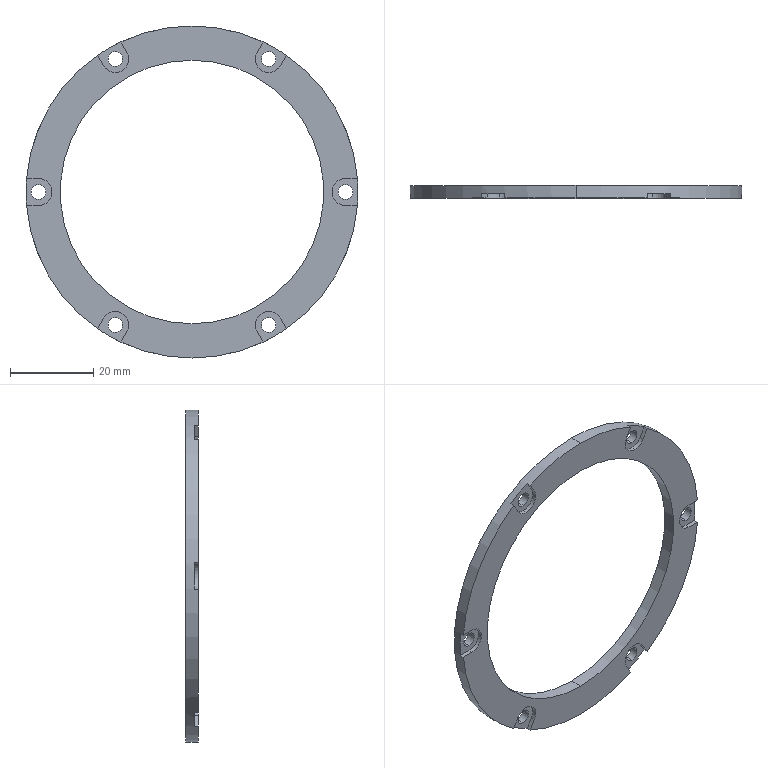Part | SolidWorks | features CirPattern 3, ICE 2, Cut 1, Extrusion 1 | 1 solid | 44 faces | box 80 x 3 x 80 mm | volume 5249 mm3 | cylinder 24 | plane 20 | commonest cylinder face diameters 3.5 x12 6.5 x8 63.5 x2 80 x2
STEP:
#1=CARTESIAN_POINT('',(0.,3.,-31.75));
#2=VERTEX_POINT('',#1);
#3=CARTESIAN_POINT('',(0.,3.,31.75));
#4=VERTEX_POINT('',#3);
#5=CARTESIAN_POINT('',(0.,3.,0.));
#6=DIRECTION('',(0.,1.,0.));
#7=DIRECTION('',(0.,0.,1.));
#8=AXIS2_PLACEMENT_3D('',#5,#6,#7);
#9=CIRCLE('',#8,31.75);
#10=EDGE_CURVE('',#2,#4,#9,.T.);
#11=ORIENTED_EDGE('',*,*,#10,.T.);
#12=CARTESIAN_POINT('',(0.,0.,31.75));
#13=VERTEX_POINT('',#12);
#14=CARTESIAN_POINT('',(0.,3.,31.75));
#15=DIRECTION('',(0.,-1.,0.));
#16=VECTOR('',#15,1000.);
#17=LINE('',#14,#16);
#18=EDGE_CURVE('',#4,#13,#17,.T.);
#19=ORIENTED_EDGE('',*,*,#18,.T.);
#20=CARTESIAN_POINT('',(0.,0.,-31.75));
#21=VERTEX_POINT('',#20);
#22=CARTESIAN_POINT('',(0.,0.,0.));
#23=DIRECTION('',(0.,1.,0.));
#24=DIRECTION('',(0.,0.,1.));
#25=AXIS2_PLACEMENT_3D('',#22,#23,#24);
#26=CIRCLE('',#25,31.75);
#27=EDGE_CURVE('',#21,#13,#26,.T.);
#28=ORIENTED_EDGE('',*,*,#27,.F.);
#29=CARTESIAN_POINT('',(0.,3.,-31.75));
#30=DIRECTION('',(0.,-1.,0.));
#31=VECTOR('',#30,1000.);
#32=LINE('',#29,#31);
#33=EDGE_CURVE('',#2,#21,#32,.T.);
#34=ORIENTED_EDGE('',*,*,#33,.F.);
#35=EDGE_LOOP('',(#11,#19,#28,#34));
#36=FACE_OUTER_BOUND('',#35,.T.);
#37=CARTESIAN_POINT('',(0.,3.,0.));
#38=DIRECTION('',(0.,-1.,0.));
#39=DIRECTION('',(0.,0.,-1.));
#40=AXIS2_PLACEMENT_3D('',#37,#38,#39);
#41=CYLINDRICAL_SURFACE('',#40,31.75);
#42=ADVANCED_FACE('',(#36),#41,.F.);
#43=CARTESIAN_POINT('',(0.,3.,40.));
#44=VERTEX_POINT('',#43);
#45=CARTESIAN_POINT('',(0.,3.,-40.));
#46=VERTEX_POINT('',#45);
#47=CARTESIAN_POINT('',(0.,3.,0.));
#48=DIRECTION('',(0.,1.,0.));
#49=DIRECTION('',(0.,0.,1.));
#50=AXIS2_PLACEMENT_3D('',#47,#48,#49);
#51=CIRCLE('',#50,40.);
#52=EDGE_CURVE('',#44,#46,#51,.T.);
#53=ORIENTED_EDGE('',*,*,#52,.F.);
#54=CARTESIAN_POINT('',(0.,0.,40.));
#55=VERTEX_POINT('',#54);
#56=CARTESIAN_POINT('',(0.,3.,40.));
#57=DIRECTION('',(0.,-1.,0.));
#58=VECTOR('',#57,1000.);
#59=LINE('',#56,#58);
#60=EDGE_CURVE('',#44,#55,#59,.T.);
#61=ORIENTED_EDGE('',*,*,#60,.T.);
#62=CARTESIAN_POINT('',(17.119,0.,36.151));
#63=VERTEX_POINT('',#62);
#64=CARTESIAN_POINT('',(0.,0.,0.));
#65=DIRECTION('',(0.,1.,0.));
#66=DIRECTION('',(0.,0.,1.));
#67=AXIS2_PLACEMENT_3D('',#64,#65,#66);
#68=CIRCLE('',#67,40.);
#69=EDGE_CURVE('',#55,#63,#68,.T.);
#70=ORIENTED_EDGE('',*,*,#69,.T.);
#71=CARTESIAN_POINT('',(17.119,1.,36.151));
#72=VERTEX_POINT('',#71);
#73=CARTESIAN_POINT('',(17.119,3.,36.151));
#74=DIRECTION('',(0.,1.,0.));
#75=VECTOR('',#74,1000.);
#76=LINE('',#73,#75);
#77=EDGE_CURVE('',#63,#72,#76,.T.);
#78=ORIENTED_EDGE('',*,*,#77,.T.);
#79=CARTESIAN_POINT('',(22.748,1.,32.901));
#80=VERTEX_POINT('',#79);
#81=CARTESIAN_POINT('',(0.,1.,0.));
#82=DIRECTION('',(0.,-1.,0.));
#83=DIRECTION('',(0.,0.,-1.));
#84=AXIS2_PLACEMENT_3D('',#81,#82,#83);
#85=CIRCLE('',#84,40.);
#86=EDGE_CURVE('',#80,#72,#85,.T.);
#87=ORIENTED_EDGE('',*,*,#86,.F.);
#88=CARTESIAN_POINT('',(22.748,0.,32.901));
#89=VERTEX_POINT('',#88);
#90=CARTESIAN_POINT('',(22.748,3.,32.901));
#91=DIRECTION('',(0.,-1.,0.));
#92=VECTOR('',#91,1000.);
#93=LINE('',#90,#92);
#94=EDGE_CURVE('',#80,#89,#93,.T.);
#95=ORIENTED_EDGE('',*,*,#94,.T.);
#96=CARTESIAN_POINT('',(39.868,0.,3.25));
#97=VERTEX_POINT('',#96);
#98=CARTESIAN_POINT('',(0.,0.,0.));
#99=DIRECTION('',(0.,1.,0.));
#100=DIRECTION('',(0.,0.,1.));
#101=AXIS2_PLACEMENT_3D('',#98,#99,#100);
#102=CIRCLE('',#101,40.);
#103=EDGE_CURVE('',#89,#97,#102,.T.);
#104=ORIENTED_EDGE('',*,*,#103,.T.);
#105=CARTESIAN_POINT('',(39.868,1.,3.25));
#106=VERTEX_POINT('',#105);
#107=CARTESIAN_POINT('',(39.868,3.,3.25));
#108=DIRECTION('',(0.,1.,0.));
#109=VECTOR('',#108,1000.);
#110=LINE('',#107,#109);
#111=EDGE_CURVE('',#97,#106,#110,.T.);
#112=ORIENTED_EDGE('',*,*,#111,.T.);
#113=CARTESIAN_POINT('',(39.868,1.,-3.25));
#114=VERTEX_POINT('',#113);
#115=CARTESIAN_POINT('',(0.,1.,0.));
#116=DIRECTION('',(0.,-1.,0.));
#117=DIRECTION('',(0.,0.,-1.));
#118=AXIS2_PLACEMENT_3D('',#115,#116,#117);
#119=CIRCLE('',#118,40.);
#120=EDGE_CURVE('',#114,#106,#119,.T.);
#121=ORIENTED_EDGE('',*,*,#120,.F.);
#122=CARTESIAN_POINT('',(39.868,0.,-3.25));
#123=VERTEX_POINT('',#122);
#124=CARTESIAN_POINT('',(39.868,3.,-3.25));
#125=DIRECTION('',(0.,-1.,0.));
#126=VECTOR('',#125,1000.);
#127=LINE('',#124,#126);
#128=EDGE_CURVE('',#114,#123,#127,.T.);
#129=ORIENTED_EDGE('',*,*,#128,.T.);
#130=CARTESIAN_POINT('',(22.748,0.,-32.901));
#131=VERTEX_POINT('',#130);
#132=CARTESIAN_POINT('',(0.,0.,0.));
#133=DIRECTION('',(0.,1.,0.));
#134=DIRECTION('',(0.,0.,1.));
#135=AXIS2_PLACEMENT_3D('',#132,#133,#134);
#136=CIRCLE('',#135,40.);
#137=EDGE_CURVE('',#123,#131,#136,.T.);
#138=ORIENTED_EDGE('',*,*,#137,.T.);
#139=CARTESIAN_POINT('',(22.748,1.,-32.901));
#140=VERTEX_POINT('',#139);
#141=CARTESIAN_POINT('',(22.748,3.,-32.901));
#142=DIRECTION('',(0.,1.,0.));
#143=VECTOR('',#142,1000.);
#144=LINE('',#141,#143);
#145=EDGE_CURVE('',#131,#140,#144,.T.);
#146=ORIENTED_EDGE('',*,*,#145,.T.);
#147=CARTESIAN_POINT('',(17.119,1.,-36.151));
#148=VERTEX_POINT('',#147);
#149=CARTESIAN_POINT('',(0.,1.,0.));
#150=DIRECTION('',(0.,-1.,0.));
#151=DIRECTION('',(0.,0.,-1.));
#152=AXIS2_PLACEMENT_3D('',#149,#150,#151);
#153=CIRCLE('',#152,40.);
#154=EDGE_CURVE('',#148,#140,#153,.T.);
#155=ORIENTED_EDGE('',*,*,#154,.F.);
#156=CARTESIAN_POINT('',(17.119,0.,-36.151));
#157=VERTEX_POINT('',#156);
#158=CARTESIAN_POINT('',(17.119,3.,-36.151));
#159=DIRECTION('',(0.,-1.,0.));
#160=VECTOR('',#159,1000.);
#161=LINE('',#158,#160);
#162=EDGE_CURVE('',#148,#157,#161,.T.);
#163=ORIENTED_EDGE('',*,*,#162,.T.);
#164=CARTESIAN_POINT('',(0.,0.,-40.));
#165=VERTEX_POINT('',#164);
#166=CARTESIAN_POINT('',(0.,0.,0.));
#167=DIRECTION('',(0.,1.,0.));
#168=DIRECTION('',(0.,0.,1.));
#169=AXIS2_PLACEMENT_3D('',#166,#167,#168);
#170=CIRCLE('',#169,40.);
#171=EDGE_CURVE('',#157,#165,#170,.T.);
#172=ORIENTED_EDGE('',*,*,#171,.T.);
#173=CARTESIAN_POINT('',(0.,3.,-40.));
#174=DIRECTION('',(0.,-1.,0.));
#175=VECTOR('',#174,1000.);
#176=LINE('',#173,#175);
#177=EDGE_CURVE('',#46,#165,#176,.T.);
#178=ORIENTED_EDGE('',*,*,#177,.F.);
#179=EDGE_LOOP('',(#53,#61,#70,#78,#87,#95,#104,#112,#121,#129,#138,#146,#155,#163,#172,#178));
#180=FACE_OUTER_BOUND('',#179,.T.);
#181=CARTESIAN_POINT('',(0.,3.,0.));
#182=DIRECTION('',(0.,-1.,0.));
#183=DIRECTION('',(0.,0.,-1.));
#184=AXIS2_PLACEMENT_3D('',#181,#182,#183);
#185=CYLINDRICAL_SURFACE('',#184,40.);
#186=ADVANCED_FACE('',(#180),#185,.T.);
#187=CARTESIAN_POINT('',(18.5,3.,33.793));
#188=VERTEX_POINT('',#187);
#189=CARTESIAN_POINT('',(18.5,3.,30.293));
#190=VERTEX_POINT('',#189);
#191=CARTESIAN_POINT('',(18.5,3.,32.043));
#192=DIRECTION('',(0.,-1.,0.));
#193=DIRECTION('',(0.866,0.,-0.5));
#194=AXIS2_PLACEMENT_3D('',#191,#192,#193);
#195=CIRCLE('',#194,1.75);
#196=EDGE_CURVE('',#188,#190,#195,.T.);
#197=ORIENTED_EDGE('',*,*,#196,.F.);
#198=CARTESIAN_POINT('',(18.5,1.,33.793));
#199=VERTEX_POINT('',#198);
#200=CARTESIAN_POINT('',(18.5,3.,33.793));
#201=DIRECTION('',(0.,-1.,0.));
#202=VECTOR('',#201,1000.);
#203=LINE('',#200,#202);
#204=EDGE_CURVE('',#188,#199,#203,.T.);
#205=ORIENTED_EDGE('',*,*,#204,.T.);
#206=CARTESIAN_POINT('',(18.5,1.,30.293));
#207=VERTEX_POINT('',#206);
#208=CARTESIAN_POINT('',(18.5,1.,32.043));
#209=DIRECTION('',(0.,1.,0.));
#210=DIRECTION('',(0.,0.,-1.));
#211=AXIS2_PLACEMENT_3D('',#208,#209,#210);
#212=CIRCLE('',#211,1.75);
#213=EDGE_CURVE('',#207,#199,#212,.T.);
#214=ORIENTED_EDGE('',*,*,#213,.F.);
#215=CARTESIAN_POINT('',(18.5,3.,30.293));
#216=DIRECTION('',(0.,-1.,0.));
#217=VECTOR('',#216,1000.);
#218=LINE('',#215,#217);
#219=EDGE_CURVE('',#190,#207,#218,.T.);
#220=ORIENTED_EDGE('',*,*,#219,.F.);
#221=EDGE_LOOP('',(#197,#205,#214,#220));
#222=FACE_OUTER_BOUND('',#221,.T.);
#223=CARTESIAN_POINT('',(18.5,3.,32.043));
#224=DIRECTION('',(0.,-1.,0.));
#225=DIRECTION('',(0.,0.,-1.));
#226=AXIS2_PLACEMENT_3D('',#223,#224,#225);
#227=CYLINDRICAL_SURFACE('',#226,1.75);
#228=ADVANCED_FACE('',(#222),#227,.F.);
#229=CARTESIAN_POINT('',(-18.5,3.,33.793));
#230=VERTEX_POINT('',#229);
#231=CARTESIAN_POINT('',(-18.5,3.,30.293));
#232=VERTEX_POINT('',#231);
#233=CARTESIAN_POINT('',(-18.5,3.,32.043));
#234=DIRECTION('',(0.,-1.,0.));
#235=DIRECTION('',(0.866,0.,0.5));
#236=AXIS2_PLACEMENT_3D('',#233,#234,#235);
#237=CIRCLE('',#236,1.75);
#238=EDGE_CURVE('',#230,#232,#237,.T.);
#239=ORIENTED_EDGE('',*,*,#238,.F.);
#240=CARTESIAN_POINT('',(-18.5,1.,33.793));
#241=VERTEX_POINT('',#240);
#242=CARTESIAN_POINT('',(-18.5,3.,33.793));
#243=DIRECTION('',(0.,-1.,0.));
#244=VECTOR('',#243,1000.);
#245=LINE('',#242,#244);
#246=EDGE_CURVE('',#230,#241,#245,.T.);
#247=ORIENTED_EDGE('',*,*,#246,.T.);
#248=CARTESIAN_POINT('',(-18.5,1.,30.293));
#249=VERTEX_POINT('',#248);
#250=CARTESIAN_POINT('',(-18.5,1.,32.043));
#251=DIRECTION('',(0.,1.,0.));
#252=DIRECTION('',(0.,0.,-1.));
#253=AXIS2_PLACEMENT_3D('',#250,#251,#252);
#254=CIRCLE('',#253,1.75);
#255=EDGE_CURVE('',#249,#241,#254,.T.);
#256=ORIENTED_EDGE('',*,*,#255,.F.);
#257=CARTESIAN_POINT('',(-18.5,3.,30.293));
#258=DIRECTION('',(0.,-1.,0.));
#259=VECTOR('',#258,1000.);
#260=LINE('',#257,#259);
#261=EDGE_CURVE('',#232,#249,#260,.T.);
#262=ORIENTED_EDGE('',*,*,#261,.F.);
#263=EDGE_LOOP('',(#239,#247,#256,#262));
#264=FACE_OUTER_BOUND('',#263,.T.);
#265=CARTESIAN_POINT('',(-18.5,3.,32.043));
#266=DIRECTION('',(0.,-1.,0.));
#267=DIRECTION('',(0.,0.,-1.));
#268=AXIS2_PLACEMENT_3D('',#265,#266,#267);
#269=CYLINDRICAL_SURFACE('',#268,1.75);
#270=ADVANCED_FACE('',(#264),#269,.F.);
#271=CARTESIAN_POINT('',(-37.,3.,1.75));
#272=VERTEX_POINT('',#271);
#273=CARTESIAN_POINT('',(-37.,3.,-1.75));
#274=VERTEX_POINT('',#273);
#275=CARTESIAN_POINT('',(-37.,3.,0.));
#276=DIRECTION('',(0.,-1.,0.));
#277=DIRECTION('',(0.,0.,1.));
#278=AXIS2_PLACEMENT_3D('',#275,#276,#277);
#279=CIRCLE('',#278,1.75);
#280=EDGE_CURVE('',#272,#274,#279,.T.);
#281=ORIENTED_EDGE('',*,*,#280,.F.);
#282=CARTESIAN_POINT('',(-37.,1.,1.75));
#283=VERTEX_POINT('',#282);
#284=CARTESIAN_POINT('',(-37.,3.,1.75));
#285=DIRECTION('',(0.,-1.,0.));
#286=VECTOR('',#285,1000.);
#287=LINE('',#284,#286);
#288=EDGE_CURVE('',#272,#283,#287,.T.);
#289=ORIENTED_EDGE('',*,*,#288,.T.);
#290=CARTESIAN_POINT('',(-37.,1.,-1.75));
#291=VERTEX_POINT('',#290);
#292=CARTESIAN_POINT('',(-37.,1.,0.));
#293=DIRECTION('',(0.,1.,0.));
#294=DIRECTION('',(0.,0.,-1.));
#295=AXIS2_PLACEMENT_3D('',#292,#293,#294);
#296=CIRCLE('',#295,1.75);
#297=EDGE_CURVE('',#291,#283,#296,.T.);
#298=ORIENTED_EDGE('',*,*,#297,.F.);
#299=CARTESIAN_POINT('',(-37.,3.,-1.75));
#300=DIRECTION('',(0.,-1.,0.));
#301=VECTOR('',#300,1000.);
#302=LINE('',#299,#301);
#303=EDGE_CURVE('',#274,#291,#302,.T.);
#304=ORIENTED_EDGE('',*,*,#303,.F.);
#305=EDGE_LOOP('',(#281,#289,#298,#304));
#306=FACE_OUTER_BOUND('',#305,.T.);
#307=CARTESIAN_POINT('',(-37.,3.,0.));
#308=DIRECTION('',(0.,-1.,0.));
#309=DIRECTION('',(0.,0.,-1.));
#310=AXIS2_PLACEMENT_3D('',#307,#308,#309);
#311=CYLINDRICAL_SURFACE('',#310,1.75);
#312=ADVANCED_FACE('',(#306),#311,.F.);
#313=CARTESIAN_POINT('',(-18.5,3.,-30.293));
#314=VERTEX_POINT('',#313);
#315=CARTESIAN_POINT('',(-18.5,3.,-33.793));
#316=VERTEX_POINT('',#315);
#317=CARTESIAN_POINT('',(-18.5,3.,-32.043));
#318=DIRECTION('',(0.,-1.,0.));
#319=DIRECTION('',(-0.866,0.,0.5));
#320=AXIS2_PLACEMENT_3D('',#317,#318,#319);
#321=CIRCLE('',#320,1.75);
#322=EDGE_CURVE('',#314,#316,#321,.T.);
#323=ORIENTED_EDGE('',*,*,#322,.F.);
#324=CARTESIAN_POINT('',(-18.5,1.,-30.293));
#325=VERTEX_POINT('',#324);
#326=CARTESIAN_POINT('',(-18.5,3.,-30.293));
#327=DIRECTION('',(0.,-1.,0.));
#328=VECTOR('',#327,1000.);
#329=LINE('',#326,#328);
#330=EDGE_CURVE('',#314,#325,#329,.T.);
#331=ORIENTED_EDGE('',*,*,#330,.T.);
#332=CARTESIAN_POINT('',(-18.5,1.,-33.793));
#333=VERTEX_POINT('',#332);
#334=CARTESIAN_POINT('',(-18.5,1.,-32.043));
#335=DIRECTION('',(0.,1.,0.));
#336=DIRECTION('',(0.,0.,-1.));
#337=AXIS2_PLACEMENT_3D('',#334,#335,#336);
#338=CIRCLE('',#337,1.75);
#339=EDGE_CURVE('',#333,#325,#338,.T.);
#340=ORIENTED_EDGE('',*,*,#339,.F.);
#341=CARTESIAN_POINT('',(-18.5,3.,-33.793));
#342=DIRECTION('',(0.,-1.,0.));
#343=VECTOR('',#342,1000.);
#344=LINE('',#341,#343);
#345=EDGE_CURVE('',#316,#333,#344,.T.);
#346=ORIENTED_EDGE('',*,*,#345,.F.);
#347=EDGE_LOOP('',(#323,#331,#340,#346));
#348=FACE_OUTER_BOUND('',#347,.T.);
#349=CARTESIAN_POINT('',(-18.5,3.,-32.043));
#350=DIRECTION('',(0.,-1.,0.));
#351=DIRECTION('',(0.,0.,-1.));
#352=AXIS2_PLACEMENT_3D('',#349,#350,#351);
#353=CYLINDRICAL_SURFACE('',#352,1.75);
#354=ADVANCED_FACE('',(#348),#353,.F.);
#355=CARTESIAN_POINT('',(18.5,3.,-30.293));
#356=VERTEX_POINT('',#355);
#357=CARTESIAN_POINT('',(18.5,3.,-33.793));
#358=VERTEX_POINT('',#357);
#359=CARTESIAN_POINT('',(18.5,3.,-32.043));
#360=DIRECTION('',(0.,-1.,0.));
#361=DIRECTION('',(-0.866,0.,-0.5));
#362=AXIS2_PLACEMENT_3D('',#359,#360,#361);
#363=CIRCLE('',#362,1.75);
#364=EDGE_CURVE('',#356,#358,#363,.T.);
#365=ORIENTED_EDGE('',*,*,#364,.F.);
#366=CARTESIAN_POINT('',(18.5,1.,-30.293));
#367=VERTEX_POINT('',#366);
#368=CARTESIAN_POINT('',(18.5,3.,-30.293));
#369=DIRECTION('',(0.,-1.,0.));
#370=VECTOR('',#369,1000.);
#371=LINE('',#368,#370);
#372=EDGE_CURVE('',#356,#367,#371,.T.);
#373=ORIENTED_EDGE('',*,*,#372,.T.);
#374=CARTESIAN_POINT('',(18.5,1.,-33.793));
#375=VERTEX_POINT('',#374);
#376=CARTESIAN_POINT('',(18.5,1.,-32.043));
#377=DIRECTION('',(0.,1.,0.));
#378=DIRECTION('',(0.,0.,-1.));
#379=AXIS2_PLACEMENT_3D('',#376,#377,#378);
#380=CIRCLE('',#379,1.75);
#381=EDGE_CURVE('',#375,#367,#380,.T.);
#382=ORIENTED_EDGE('',*,*,#381,.F.);
#383=CARTESIAN_POINT('',(18.5,3.,-33.793));
#384=DIRECTION('',(0.,-1.,0.));
#385=VECTOR('',#384,1000.);
#386=LINE('',#383,#385);
#387=EDGE_CURVE('',#358,#375,#386,.T.);
#388=ORIENTED_EDGE('',*,*,#387,.F.);
#389=EDGE_LOOP('',(#365,#373,#382,#388));
#390=FACE_OUTER_BOUND('',#389,.T.);
#391=CARTESIAN_POINT('',(18.5,3.,-32.043));
#392=DIRECTION('',(0.,-1.,0.));
#393=DIRECTION('',(0.,0.,-1.));
#394=AXIS2_PLACEMENT_3D('',#391,#392,#393);
#395=CYLINDRICAL_SURFACE('',#394,1.75);
#396=ADVANCED_FACE('',(#390),#395,.F.);
#397=CARTESIAN_POINT('',(37.,3.,1.75));
#398=VERTEX_POINT('',#397);
#399=CARTESIAN_POINT('',(37.,3.,-1.75));
#400=VERTEX_POINT('',#399);
#401=CARTESIAN_POINT('',(37.,3.,0.));
#402=DIRECTION('',(0.,-1.,0.));
#403=DIRECTION('',(0.,0.,-1.));
#404=AXIS2_PLACEMENT_3D('',#401,#402,#403);
#405=CIRCLE('',#404,1.75);
#406=EDGE_CURVE('',#398,#400,#405,.T.);
#407=ORIENTED_EDGE('',*,*,#406,.F.);
#408=CARTESIAN_POINT('',(37.,1.,1.75));
#409=VERTEX_POINT('',#408);
#410=CARTESIAN_POINT('',(37.,3.,1.75));
#411=DIRECTION('',(0.,-1.,0.));
#412=VECTOR('',#411,1000.);
#413=LINE('',#410,#412);
#414=EDGE_CURVE('',#398,#409,#413,.T.);
#415=ORIENTED_EDGE('',*,*,#414,.T.);
#416=CARTESIAN_POINT('',(37.,1.,-1.75));
#417=VERTEX_POINT('',#416);
#418=CARTESIAN_POINT('',(37.,1.,0.));
#419=DIRECTION('',(0.,1.,0.));
#420=DIRECTION('',(0.,0.,-1.));
#421=AXIS2_PLACEMENT_3D('',#418,#419,#420);
#422=CIRCLE('',#421,1.75);
#423=EDGE_CURVE('',#417,#409,#422,.T.);
#424=ORIENTED_EDGE('',*,*,#423,.F.);
#425=CARTESIAN_POINT('',(37.,3.,-1.75));
#426=DIRECTION('',(0.,-1.,0.));
#427=VECTOR('',#426,1000.);
#428=LINE('',#425,#427);
#429=EDGE_CURVE('',#400,#417,#428,.T.);
#430=ORIENTED_EDGE('',*,*,#429,.F.);
#431=EDGE_LOOP('',(#407,#415,#424,#430));
#432=FACE_OUTER_BOUND('',#431,.T.);
#433=CARTESIAN_POINT('',(37.,3.,0.));
#434=DIRECTION('',(0.,-1.,0.));
#435=DIRECTION('',(0.,0.,-1.));
#436=AXIS2_PLACEMENT_3D('',#433,#434,#435);
#437=CYLINDRICAL_SURFACE('',#436,1.75);
#438=ADVANCED_FACE('',(#432),#437,.F.);
#439=CARTESIAN_POINT('',(18.5,1.,28.793));
#440=VERTEX_POINT('',#439);
#441=CARTESIAN_POINT('',(21.315,1.,30.418));
#442=VERTEX_POINT('',#441);
#443=CARTESIAN_POINT('',(18.5,1.,32.043));
#444=DIRECTION('',(0.,-1.,0.));
#445=DIRECTION('',(0.,0.,-1.));
#446=AXIS2_PLACEMENT_3D('',#443,#444,#445);
#447=CIRCLE('',#446,3.25);
#448=EDGE_CURVE('',#440,#442,#447,.T.);
#449=ORIENTED_EDGE('',*,*,#448,.F.);
#450=CARTESIAN_POINT('',(18.5,0.,28.793));
#451=VERTEX_POINT('',#450);
#452=CARTESIAN_POINT('',(18.5,1.,28.793));
#453=DIRECTION('',(0.,-1.,0.));
#454=VECTOR('',#453,1000.);
#455=LINE('',#452,#454);
#456=EDGE_CURVE('',#440,#451,#455,.T.);
#457=ORIENTED_EDGE('',*,*,#456,.T.);
#458=CARTESIAN_POINT('',(21.315,0.,30.418));
#459=VERTEX_POINT('',#458);
#460=CARTESIAN_POINT('',(18.5,0.,32.043));
#461=DIRECTION('',(0.,-1.,0.));
#462=DIRECTION('',(0.,0.,-1.));
#463=AXIS2_PLACEMENT_3D('',#460,#461,#462);
#464=CIRCLE('',#463,3.25);
#465=EDGE_CURVE('',#451,#459,#464,.T.);
#466=ORIENTED_EDGE('',*,*,#465,.T.);
#467=CARTESIAN_POINT('',(21.315,10.69,30.418));
#468=DIRECTION('',(0.,-1.,0.));
#469=VECTOR('',#468,1000.);
#470=LINE('',#467,#469);
#471=EDGE_CURVE('',#442,#459,#470,.T.);
#472=ORIENTED_EDGE('',*,*,#471,.F.);
#473=EDGE_LOOP('',(#449,#457,#466,#472));
#474=FACE_OUTER_BOUND('',#473,.T.);
#475=CARTESIAN_POINT('',(18.5,1.,32.043));
#476=DIRECTION('',(0.,-1.,0.));
#477=DIRECTION('',(0.,0.,-1.));
#478=AXIS2_PLACEMENT_3D('',#475,#476,#477);
#479=CYLINDRICAL_SURFACE('',#478,3.25);
#480=ADVANCED_FACE('',(#474),#479,.F.);
#481=CARTESIAN_POINT('',(-18.5,1.,28.793));
#482=VERTEX_POINT('',#481);
#483=CARTESIAN_POINT('',(-15.685,1.,33.668));
#484=VERTEX_POINT('',#483);
#485=CARTESIAN_POINT('',(-18.5,1.,32.043));
#486=DIRECTION('',(0.,-1.,0.));
#487=DIRECTION('',(0.866,0.,-0.5));
#488=AXIS2_PLACEMENT_3D('',#485,#486,#487);
#489=CIRCLE('',#488,3.25);
#490=EDGE_CURVE('',#482,#484,#489,.T.);
#491=ORIENTED_EDGE('',*,*,#490,.F.);
#492=CARTESIAN_POINT('',(-18.5,0.,28.793));
#493=VERTEX_POINT('',#492);
#494=CARTESIAN_POINT('',(-18.5,1.,28.793));
#495=DIRECTION('',(0.,-1.,0.));
#496=VECTOR('',#495,1000.);
#497=LINE('',#494,#496);
#498=EDGE_CURVE('',#482,#493,#497,.T.);
#499=ORIENTED_EDGE('',*,*,#498,.T.);
#500=CARTESIAN_POINT('',(-15.685,0.,33.668));
#501=VERTEX_POINT('',#500);
#502=CARTESIAN_POINT('',(-18.5,0.,32.043));
#503=DIRECTION('',(0.,-1.,0.));
#504=DIRECTION('',(0.866,0.,-0.5));
#505=AXIS2_PLACEMENT_3D('',#502,#503,#504);
#506=CIRCLE('',#505,3.25);
#507=EDGE_CURVE('',#493,#501,#506,.T.);
#508=ORIENTED_EDGE('',*,*,#507,.T.);
#509=CARTESIAN_POINT('',(-15.685,10.69,33.668));
#510=DIRECTION('',(0.,-1.,0.));
#511=VECTOR('',#510,1000.);
#512=LINE('',#509,#511);
#513=EDGE_CURVE('',#484,#501,#512,.T.);
#514=ORIENTED_EDGE('',*,*,#513,.F.);
#515=EDGE_LOOP('',(#491,#499,#508,#514));
#516=FACE_OUTER_BOUND('',#515,.T.);
#517=CARTESIAN_POINT('',(-18.5,1.,32.043));
#518=DIRECTION('',(0.,-1.,0.));
#519=DIRECTION('',(0.,0.,-1.));
#520=AXIS2_PLACEMENT_3D('',#517,#518,#519);
#521=CYLINDRICAL_SURFACE('',#520,3.25);
#522=ADVANCED_FACE('',(#516),#521,.F.);
#523=CARTESIAN_POINT('',(21.315,1.,-30.418));
#524=VERTEX_POINT('',#523);
#525=CARTESIAN_POINT('',(21.315,0.,-30.418));
#526=VERTEX_POINT('',#525);
#527=CARTESIAN_POINT('',(21.315,10.69,-30.418));
#528=DIRECTION('',(0.,-1.,0.));
#529=VECTOR('',#528,1000.);
#530=LINE('',#527,#529);
#531=EDGE_CURVE('',#524,#526,#530,.T.);
#532=ORIENTED_EDGE('',*,*,#531,.T.);
#533=CARTESIAN_POINT('',(15.685,0.,-33.668));
#534=VERTEX_POINT('',#533);
#535=CARTESIAN_POINT('',(18.5,0.,-32.043));
#536=DIRECTION('',(0.,-1.,0.));
#537=DIRECTION('',(-0.866,0.,0.5));
#538=AXIS2_PLACEMENT_3D('',#535,#536,#537);
#539=CIRCLE('',#538,3.25);
#540=EDGE_CURVE('',#526,#534,#539,.T.);
#541=ORIENTED_EDGE('',*,*,#540,.T.);
#542=CARTESIAN_POINT('',(15.685,1.,-33.668));
#543=VERTEX_POINT('',#542);
#544=CARTESIAN_POINT('',(15.685,10.69,-33.668));
#545=DIRECTION('',(0.,-1.,0.));
#546=VECTOR('',#545,1000.);
#547=LINE('',#544,#546);
#548=EDGE_CURVE('',#543,#534,#547,.T.);
#549=ORIENTED_EDGE('',*,*,#548,.F.);
#550=CARTESIAN_POINT('',(18.5,1.,-32.043));
#551=DIRECTION('',(0.,-1.,0.));
#552=DIRECTION('',(-0.866,0.,0.5));
#553=AXIS2_PLACEMENT_3D('',#550,#551,#552);
#554=CIRCLE('',#553,3.25);
#555=EDGE_CURVE('',#524,#543,#554,.T.);
#556=ORIENTED_EDGE('',*,*,#555,.F.);
#557=EDGE_LOOP('',(#532,#541,#549,#556));
#558=FACE_OUTER_BOUND('',#557,.T.);
#559=CARTESIAN_POINT('',(18.5,1.,-32.043));
#560=DIRECTION('',(0.,-1.,0.));
#561=DIRECTION('',(0.,0.,-1.));
#562=AXIS2_PLACEMENT_3D('',#559,#560,#561);
#563=CYLINDRICAL_SURFACE('',#562,3.25);
#564=ADVANCED_FACE('',(#558),#563,.F.);
#565=CARTESIAN_POINT('',(-15.685,1.,-33.668));
#566=VERTEX_POINT('',#565);
#567=CARTESIAN_POINT('',(-15.685,0.,-33.668));
#568=VERTEX_POINT('',#567);
#569=CARTESIAN_POINT('',(-15.685,10.69,-33.668));
#570=DIRECTION('',(0.,-1.,0.));
#571=VECTOR('',#570,1000.);
#572=LINE('',#569,#571);
#573=EDGE_CURVE('',#566,#568,#572,.T.);
#574=ORIENTED_EDGE('',*,*,#573,.T.);
#575=CARTESIAN_POINT('',(-21.315,0.,-30.418));
#576=VERTEX_POINT('',#575);
#577=CARTESIAN_POINT('',(-18.5,0.,-32.043));
#578=DIRECTION('',(0.,-1.,0.));
#579=DIRECTION('',(0.,0.,1.));
#580=AXIS2_PLACEMENT_3D('',#577,#578,#579);
#581=CIRCLE('',#580,3.25);
#582=EDGE_CURVE('',#568,#576,#581,.T.);
#583=ORIENTED_EDGE('',*,*,#582,.T.);
#584=CARTESIAN_POINT('',(-21.315,1.,-30.418));
#585=VERTEX_POINT('',#584);
#586=CARTESIAN_POINT('',(-21.315,10.69,-30.418));
#587=DIRECTION('',(0.,-1.,0.));
#588=VECTOR('',#587,1000.);
#589=LINE('',#586,#588);
#590=EDGE_CURVE('',#585,#576,#589,.T.);
#591=ORIENTED_EDGE('',*,*,#590,.F.);
#592=CARTESIAN_POINT('',(-18.5,1.,-32.043));
#593=DIRECTION('',(0.,-1.,0.));
#594=DIRECTION('',(0.,0.,1.));
#595=AXIS2_PLACEMENT_3D('',#592,#593,#594);
#596=CIRCLE('',#595,3.25);
#597=EDGE_CURVE('',#566,#585,#596,.T.);
#598=ORIENTED_EDGE('',*,*,#597,.F.);
#599=EDGE_LOOP('',(#574,#583,#591,#598));
#600=FACE_OUTER_BOUND('',#599,.T.);
#601=CARTESIAN_POINT('',(-18.5,1.,-32.043));
#602=DIRECTION('',(0.,-1.,0.));
#603=DIRECTION('',(0.,0.,-1.));
#604=AXIS2_PLACEMENT_3D('',#601,#602,#603);
#605=CYLINDRICAL_SURFACE('',#604,3.25);
#606=ADVANCED_FACE('',(#600),#605,.F.);
#607=CARTESIAN_POINT('',(-37.,1.,-3.25));
#608=VERTEX_POINT('',#607);
#609=CARTESIAN_POINT('',(-37.,0.,-3.25));
#610=VERTEX_POINT('',#609);
#611=CARTESIAN_POINT('',(-37.,8.382,-3.25));
#612=DIRECTION('',(0.,-1.,0.));
#613=VECTOR('',#612,1000.);
#614=LINE('',#611,#613);
#615=EDGE_CURVE('',#608,#610,#614,.T.);
#616=ORIENTED_EDGE('',*,*,#615,.T.);
#617=CARTESIAN_POINT('',(-37.,0.,3.25));
#618=VERTEX_POINT('',#617);
#619=CARTESIAN_POINT('',(-37.,0.,0.));
#620=DIRECTION('',(0.,-1.,0.));
#621=DIRECTION('',(0.866,0.,0.5));
#622=AXIS2_PLACEMENT_3D('',#619,#620,#621);
#623=CIRCLE('',#622,3.25);
#624=EDGE_CURVE('',#610,#618,#623,.T.);
#625=ORIENTED_EDGE('',*,*,#624,.T.);
#626=CARTESIAN_POINT('',(-37.,1.,3.25));
#627=VERTEX_POINT('',#626);
#628=CARTESIAN_POINT('',(-37.,8.382,3.25));
#629=DIRECTION('',(0.,-1.,0.));
#630=VECTOR('',#629,1000.);
#631=LINE('',#628,#630);
#632=EDGE_CURVE('',#627,#618,#631,.T.);
#633=ORIENTED_EDGE('',*,*,#632,.F.);
#634=CARTESIAN_POINT('',(-37.,1.,0.));
#635=DIRECTION('',(0.,-1.,0.));
#636=DIRECTION('',(0.866,0.,0.5));
#637=AXIS2_PLACEMENT_3D('',#634,#635,#636);
#638=CIRCLE('',#637,3.25);
#639=EDGE_CURVE('',#608,#627,#638,.T.);
#640=ORIENTED_EDGE('',*,*,#639,.F.);
#641=EDGE_LOOP('',(#616,#625,#633,#640));
#642=FACE_OUTER_BOUND('',#641,.T.);
#643=CARTESIAN_POINT('',(-37.,1.,0.));
#644=DIRECTION('',(0.,-1.,0.));
#645=DIRECTION('',(0.,0.,-1.));
#646=AXIS2_PLACEMENT_3D('',#643,#644,#645);
#647=CYLINDRICAL_SURFACE('',#646,3.25);
#648=ADVANCED_FACE('',(#642),#647,.F.);
#649=ORIENTED_EDGE('',*,*,#498,.F.);
#650=CARTESIAN_POINT('',(-21.315,1.,30.418));
#651=VERTEX_POINT('',#650);
#652=CARTESIAN_POINT('',(-18.5,1.,32.043));
#653=DIRECTION('',(0.,-1.,0.));
#654=DIRECTION('',(0.866,0.,-0.5));
#655=AXIS2_PLACEMENT_3D('',#652,#653,#654);
#656=CIRCLE('',#655,3.25);
#657=EDGE_CURVE('',#651,#482,#656,.T.);
#658=ORIENTED_EDGE('',*,*,#657,.F.);
#659=CARTESIAN_POINT('',(-21.315,0.,30.418));
#660=VERTEX_POINT('',#659);
#661=CARTESIAN_POINT('',(-21.315,10.69,30.418));
#662=DIRECTION('',(0.,-1.,0.));
#663=VECTOR('',#662,1000.);
#664=LINE('',#661,#663);
#665=EDGE_CURVE('',#651,#660,#664,.T.);
#666=ORIENTED_EDGE('',*,*,#665,.T.);
#667=CARTESIAN_POINT('',(-18.5,0.,32.043));
#668=DIRECTION('',(0.,-1.,0.));
#669=DIRECTION('',(0.866,0.,-0.5));
#670=AXIS2_PLACEMENT_3D('',#667,#668,#669);
#671=CIRCLE('',#670,3.25);
#672=EDGE_CURVE('',#660,#493,#671,.T.);
#673=ORIENTED_EDGE('',*,*,#672,.T.);
#674=EDGE_LOOP('',(#649,#658,#666,#673));
#675=FACE_OUTER_BOUND('',#674,.T.);
#676=CARTESIAN_POINT('',(-18.5,1.,32.043));
#677=DIRECTION('',(0.,-1.,0.));
#678=DIRECTION('',(0.,0.,-1.));
#679=AXIS2_PLACEMENT_3D('',#676,#677,#678);
#680=CYLINDRICAL_SURFACE('',#679,3.25);
#681=ADVANCED_FACE('',(#675),#680,.F.);
#682=ORIENTED_EDGE('',*,*,#456,.F.);
#683=CARTESIAN_POINT('',(15.685,1.,33.668));
#684=VERTEX_POINT('',#683);
#685=CARTESIAN_POINT('',(18.5,1.,32.043));
#686=DIRECTION('',(0.,-1.,0.));
#687=DIRECTION('',(0.,0.,-1.));
#688=AXIS2_PLACEMENT_3D('',#685,#686,#687);
#689=CIRCLE('',#688,3.25);
#690=EDGE_CURVE('',#684,#440,#689,.T.);
#691=ORIENTED_EDGE('',*,*,#690,.F.);
#692=CARTESIAN_POINT('',(15.685,0.,33.668));
#693=VERTEX_POINT('',#692);
#694=CARTESIAN_POINT('',(15.685,10.69,33.668));
#695=DIRECTION('',(0.,-1.,0.));
#696=VECTOR('',#695,1000.);
#697=LINE('',#694,#696);
#698=EDGE_CURVE('',#684,#693,#697,.T.);
#699=ORIENTED_EDGE('',*,*,#698,.T.);
#700=CARTESIAN_POINT('',(18.5,0.,32.043));
#701=DIRECTION('',(0.,-1.,0.));
#702=DIRECTION('',(0.,0.,-1.));
#703=AXIS2_PLACEMENT_3D('',#700,#701,#702);
#704=CIRCLE('',#703,3.25);
#705=EDGE_CURVE('',#693,#451,#704,.T.);
#706=ORIENTED_EDGE('',*,*,#705,.T.);
#707=EDGE_LOOP('',(#682,#691,#699,#706));
#708=FACE_OUTER_BOUND('',#707,.T.);
#709=CARTESIAN_POINT('',(18.5,1.,32.043));
#710=DIRECTION('',(0.,-1.,0.));
#711=DIRECTION('',(0.,0.,-1.));
#712=AXIS2_PLACEMENT_3D('',#709,#710,#711);
#713=CYLINDRICAL_SURFACE('',#712,3.25);
#714=ADVANCED_FACE('',(#708),#713,.F.);
#715=CARTESIAN_POINT('',(37.,1.,3.25));
#716=VERTEX_POINT('',#715);
#717=CARTESIAN_POINT('',(37.,0.,3.25));
#718=VERTEX_POINT('',#717);
#719=CARTESIAN_POINT('',(37.,8.382,3.25));
#720=DIRECTION('',(0.,-1.,0.));
#721=VECTOR('',#720,1000.);
#722=LINE('',#719,#721);
#723=EDGE_CURVE('',#716,#718,#722,.T.);
#724=ORIENTED_EDGE('',*,*,#723,.T.);
#725=CARTESIAN_POINT('',(37.,0.,-3.25));
#726=VERTEX_POINT('',#725);
#727=CARTESIAN_POINT('',(37.,0.,0.));
#728=DIRECTION('',(0.,-1.,0.));
#729=DIRECTION('',(-0.866,0.,-0.5));
#730=AXIS2_PLACEMENT_3D('',#727,#728,#729);
#731=CIRCLE('',#730,3.25);
#732=EDGE_CURVE('',#718,#726,#731,.T.);
#733=ORIENTED_EDGE('',*,*,#732,.T.);
#734=CARTESIAN_POINT('',(37.,1.,-3.25));
#735=VERTEX_POINT('',#734);
#736=CARTESIAN_POINT('',(37.,8.382,-3.25));
#737=DIRECTION('',(0.,-1.,0.));
#738=VECTOR('',#737,1000.);
#739=LINE('',#736,#738);
#740=EDGE_CURVE('',#735,#726,#739,.T.);
#741=ORIENTED_EDGE('',*,*,#740,.F.);
#742=CARTESIAN_POINT('',(37.,1.,0.));
#743=DIRECTION('',(0.,-1.,0.));
#744=DIRECTION('',(-0.866,0.,-0.5));
#745=AXIS2_PLACEMENT_3D('',#742,#743,#744);
#746=CIRCLE('',#745,3.25);
#747=EDGE_CURVE('',#716,#735,#746,.T.);
#748=ORIENTED_EDGE('',*,*,#747,.F.);
#749=EDGE_LOOP('',(#724,#733,#741,#748));
#750=FACE_OUTER_BOUND('',#749,.T.);
#751=CARTESIAN_POINT('',(37.,1.,0.));
#752=DIRECTION('',(0.,-1.,0.));
#753=DIRECTION('',(0.,0.,-1.));
#754=AXIS2_PLACEMENT_3D('',#751,#752,#753);
#755=CYLINDRICAL_SURFACE('',#754,3.25);
#756=ADVANCED_FACE('',(#750),#755,.F.);
#757=ORIENTED_EDGE('',*,*,#414,.F.);
#758=CARTESIAN_POINT('',(37.,3.,0.));
#759=DIRECTION('',(0.,-1.,0.));
#760=DIRECTION('',(0.,0.,-1.));
#761=AXIS2_PLACEMENT_3D('',#758,#759,#760);
#762=CIRCLE('',#761,1.75);
#763=EDGE_CURVE('',#400,#398,#762,.T.);
#764=ORIENTED_EDGE('',*,*,#763,.F.);
#765=ORIENTED_EDGE('',*,*,#429,.T.);
#766=CARTESIAN_POINT('',(37.,1.,0.));
#767=DIRECTION('',(0.,1.,0.));
#768=DIRECTION('',(0.,0.,-1.));
#769=AXIS2_PLACEMENT_3D('',#766,#767,#768);
#770=CIRCLE('',#769,1.75);
#771=EDGE_CURVE('',#409,#417,#770,.T.);
#772=ORIENTED_EDGE('',*,*,#771,.F.);
#773=EDGE_LOOP('',(#757,#764,#765,#772));
#774=FACE_OUTER_BOUND('',#773,.T.);
#775=CARTESIAN_POINT('',(37.,3.,0.));
#776=DIRECTION('',(0.,-1.,0.));
#777=DIRECTION('',(0.,0.,-1.));
#778=AXIS2_PLACEMENT_3D('',#775,#776,#777);
#779=CYLINDRICAL_SURFACE('',#778,1.75);
#780=ADVANCED_FACE('',(#774),#779,.F.);
#781=ORIENTED_EDGE('',*,*,#372,.F.);
#782=CARTESIAN_POINT('',(18.5,3.,-32.043));
#783=DIRECTION('',(0.,-1.,0.));
#784=DIRECTION('',(-0.866,0.,-0.5));
#785=AXIS2_PLACEMENT_3D('',#782,#783,#784);
#786=CIRCLE('',#785,1.75);
#787=EDGE_CURVE('',#358,#356,#786,.T.);
#788=ORIENTED_EDGE('',*,*,#787,.F.);
#789=ORIENTED_EDGE('',*,*,#387,.T.);
#790=CARTESIAN_POINT('',(18.5,1.,-32.043));
#791=DIRECTION('',(0.,1.,0.));
#792=DIRECTION('',(0.,0.,-1.));
#793=AXIS2_PLACEMENT_3D('',#790,#791,#792);
#794=CIRCLE('',#793,1.75);
#795=EDGE_CURVE('',#367,#375,#794,.T.);
#796=ORIENTED_EDGE('',*,*,#795,.F.);
#797=EDGE_LOOP('',(#781,#788,#789,#796));
#798=FACE_OUTER_BOUND('',#797,.T.);
#799=CARTESIAN_POINT('',(18.5,3.,-32.043));
#800=DIRECTION('',(0.,-1.,0.));
#801=DIRECTION('',(0.,0.,-1.));
#802=AXIS2_PLACEMENT_3D('',#799,#800,#801);
#803=CYLINDRICAL_SURFACE('',#802,1.75);
#804=ADVANCED_FACE('',(#798),#803,.F.);
#805=ORIENTED_EDGE('',*,*,#330,.F.);
#806=CARTESIAN_POINT('',(-18.5,3.,-32.043));
#807=DIRECTION('',(0.,-1.,0.));
#808=DIRECTION('',(-0.866,0.,0.5));
#809=AXIS2_PLACEMENT_3D('',#806,#807,#808);
#810=CIRCLE('',#809,1.75);
#811=EDGE_CURVE('',#316,#314,#810,.T.);
#812=ORIENTED_EDGE('',*,*,#811,.F.);
#813=ORIENTED_EDGE('',*,*,#345,.T.);
#814=CARTESIAN_POINT('',(-18.5,1.,-32.043));
#815=DIRECTION('',(0.,1.,0.));
#816=DIRECTION('',(0.,0.,-1.));
#817=AXIS2_PLACEMENT_3D('',#814,#815,#816);
#818=CIRCLE('',#817,1.75);
#819=EDGE_CURVE('',#325,#333,#818,.T.);
#820=ORIENTED_EDGE('',*,*,#819,.F.);
#821=EDGE_LOOP('',(#805,#812,#813,#820));
#822=FACE_OUTER_BOUND('',#821,.T.);
#823=CARTESIAN_POINT('',(-18.5,3.,-32.043));
#824=DIRECTION('',(0.,-1.,0.));
#825=DIRECTION('',(0.,0.,-1.));
#826=AXIS2_PLACEMENT_3D('',#823,#824,#825);
#827=CYLINDRICAL_SURFACE('',#826,1.75);
#828=ADVANCED_FACE('',(#822),#827,.F.);
#829=ORIENTED_EDGE('',*,*,#288,.F.);
#830=CARTESIAN_POINT('',(-37.,3.,0.));
#831=DIRECTION('',(0.,-1.,0.));
#832=DIRECTION('',(0.,0.,1.));
#833=AXIS2_PLACEMENT_3D('',#830,#831,#832);
#834=CIRCLE('',#833,1.75);
#835=EDGE_CURVE('',#274,#272,#834,.T.);
#836=ORIENTED_EDGE('',*,*,#835,.F.);
#837=ORIENTED_EDGE('',*,*,#303,.T.);
#838=CARTESIAN_POINT('',(-37.,1.,0.));
#839=DIRECTION('',(0.,1.,0.));
#840=DIRECTION('',(0.,0.,-1.));
#841=AXIS2_PLACEMENT_3D('',#838,#839,#840);
#842=CIRCLE('',#841,1.75);
#843=EDGE_CURVE('',#283,#291,#842,.T.);
#844=ORIENTED_EDGE('',*,*,#843,.F.);
#845=EDGE_LOOP('',(#829,#836,#837,#844));
#846=FACE_OUTER_BOUND('',#845,.T.);
#847=CARTESIAN_POINT('',(-37.,3.,0.));
#848=DIRECTION('',(0.,-1.,0.));
#849=DIRECTION('',(0.,0.,-1.));
#850=AXIS2_PLACEMENT_3D('',#847,#848,#849);
#851=CYLINDRICAL_SURFACE('',#850,1.75);
#852=ADVANCED_FACE('',(#846),#851,.F.);
#853=ORIENTED_EDGE('',*,*,#246,.F.);
#854=CARTESIAN_POINT('',(-18.5,3.,32.043));
#855=DIRECTION('',(0.,-1.,0.));
#856=DIRECTION('',(0.866,0.,0.5));
#857=AXIS2_PLACEMENT_3D('',#854,#855,#856);
#858=CIRCLE('',#857,1.75);
#859=EDGE_CURVE('',#232,#230,#858,.T.);
#860=ORIENTED_EDGE('',*,*,#859,.F.);
#861=ORIENTED_EDGE('',*,*,#261,.T.);
#862=CARTESIAN_POINT('',(-18.5,1.,32.043));
#863=DIRECTION('',(0.,1.,0.));
#864=DIRECTION('',(0.,0.,-1.));
#865=AXIS2_PLACEMENT_3D('',#862,#863,#864);
#866=CIRCLE('',#865,1.75);
#867=EDGE_CURVE('',#241,#249,#866,.T.);
#868=ORIENTED_EDGE('',*,*,#867,.F.);
#869=EDGE_LOOP('',(#853,#860,#861,#868));
#870=FACE_OUTER_BOUND('',#869,.T.);
#871=CARTESIAN_POINT('',(-18.5,3.,32.043));
#872=DIRECTION('',(0.,-1.,0.));
#873=DIRECTION('',(0.,0.,-1.));
#874=AXIS2_PLACEMENT_3D('',#871,#872,#873);
#875=CYLINDRICAL_SURFACE('',#874,1.75);
#876=ADVANCED_FACE('',(#870),#875,.F.);
#877=ORIENTED_EDGE('',*,*,#204,.F.);
#878=CARTESIAN_POINT('',(18.5,3.,32.043));
#879=DIRECTION('',(0.,-1.,0.));
#880=DIRECTION('',(0.866,0.,-0.5));
#881=AXIS2_PLACEMENT_3D('',#878,#879,#880);
#882=CIRCLE('',#881,1.75);
#883=EDGE_CURVE('',#190,#188,#882,.T.);
#884=ORIENTED_EDGE('',*,*,#883,.F.);
#885=ORIENTED_EDGE('',*,*,#219,.T.);
#886=CARTESIAN_POINT('',(18.5,1.,32.043));
#887=DIRECTION('',(0.,1.,0.));
#888=DIRECTION('',(0.,0.,-1.));
#889=AXIS2_PLACEMENT_3D('',#886,#887,#888);
#890=CIRCLE('',#889,1.75);
#891=EDGE_CURVE('',#199,#207,#890,.T.);
#892=ORIENTED_EDGE('',*,*,#891,.F.);
#893=EDGE_LOOP('',(#877,#884,#885,#892));
#894=FACE_OUTER_BOUND('',#893,.T.);
#895=CARTESIAN_POINT('',(18.5,3.,32.043));
#896=DIRECTION('',(0.,-1.,0.));
#897=DIRECTION('',(0.,0.,-1.));
#898=AXIS2_PLACEMENT_3D('',#895,#896,#897);
#899=CYLINDRICAL_SURFACE('',#898,1.75);
#900=ADVANCED_FACE('',(#894),#899,.F.);
#901=ORIENTED_EDGE('',*,*,#787,.T.);
#902=ORIENTED_EDGE('',*,*,#364,.T.);
#903=EDGE_LOOP('',(#901,#902));
#904=FACE_BOUND('',#903,.T.);
#905=ORIENTED_EDGE('',*,*,#811,.T.);
#906=ORIENTED_EDGE('',*,*,#322,.T.);
#907=EDGE_LOOP('',(#905,#906));
#908=FACE_BOUND('',#907,.T.);
#909=ORIENTED_EDGE('',*,*,#835,.T.);
#910=ORIENTED_EDGE('',*,*,#280,.T.);
#911=EDGE_LOOP('',(#909,#910));
#912=FACE_BOUND('',#911,.T.);
#913=ORIENTED_EDGE('',*,*,#859,.T.);
#914=ORIENTED_EDGE('',*,*,#238,.T.);
#915=EDGE_LOOP('',(#913,#914));
#916=FACE_BOUND('',#915,.T.);
#917=ORIENTED_EDGE('',*,*,#883,.T.);
#918=ORIENTED_EDGE('',*,*,#196,.T.);
#919=EDGE_LOOP('',(#917,#918));
#920=FACE_BOUND('',#919,.T.);
#921=ORIENTED_EDGE('',*,*,#763,.T.);
#922=ORIENTED_EDGE('',*,*,#406,.T.);
#923=EDGE_LOOP('',(#921,#922));
#924=FACE_BOUND('',#923,.T.);
#925=CARTESIAN_POINT('',(0.,3.,0.));
#926=DIRECTION('',(0.,1.,0.));
#927=DIRECTION('',(0.,0.,1.));
#928=AXIS2_PLACEMENT_3D('',#925,#926,#927);
#929=CIRCLE('',#928,40.);
#930=EDGE_CURVE('',#46,#44,#929,.T.);
#931=ORIENTED_EDGE('',*,*,#930,.T.);
#932=ORIENTED_EDGE('',*,*,#52,.T.);
#933=EDGE_LOOP('',(#931,#932));
#934=FACE_OUTER_BOUND('',#933,.T.);
#935=ORIENTED_EDGE('',*,*,#10,.F.);
#936=CARTESIAN_POINT('',(0.,3.,0.));
#937=DIRECTION('',(0.,1.,0.));
#938=DIRECTION('',(0.,0.,1.));
#939=AXIS2_PLACEMENT_3D('',#936,#937,#938);
#940=CIRCLE('',#939,31.75);
#941=EDGE_CURVE('',#4,#2,#940,.T.);
#942=ORIENTED_EDGE('',*,*,#941,.F.);
#943=EDGE_LOOP('',(#935,#942));
#944=FACE_BOUND('',#943,.T.);
#945=CARTESIAN_POINT('',(0.,3.,0.));
#946=DIRECTION('',(0.,1.,0.));
#947=DIRECTION('',(0.,0.,1.));
#948=AXIS2_PLACEMENT_3D('',#945,#946,#947);
#949=PLANE('',#948);
#950=ADVANCED_FACE('',(#904,#908,#912,#916,#920,#924,#934,#944),#949,.T.);
#951=ORIENTED_EDGE('',*,*,#540,.F.);
#952=CARTESIAN_POINT('',(23.065,0.,-33.449));
#953=DIRECTION('',(-0.5,0.,0.866));
#954=VECTOR('',#953,1000.);
#955=LINE('',#952,#954);
#956=EDGE_CURVE('',#131,#526,#955,.T.);
#957=ORIENTED_EDGE('',*,*,#956,.F.);
#958=ORIENTED_EDGE('',*,*,#137,.F.);
#959=CARTESIAN_POINT('',(40.5,0.,-3.25));
#960=DIRECTION('',(1.,0.,0.));
#961=VECTOR('',#960,1000.);
#962=LINE('',#959,#961);
#963=EDGE_CURVE('',#726,#123,#962,.T.);
#964=ORIENTED_EDGE('',*,*,#963,.F.);
#965=ORIENTED_EDGE('',*,*,#732,.F.);
#966=CARTESIAN_POINT('',(40.5,0.,3.25));
#967=DIRECTION('',(-1.,0.,0.));
#968=VECTOR('',#967,1000.);
#969=LINE('',#966,#968);
#970=EDGE_CURVE('',#97,#718,#969,.T.);
#971=ORIENTED_EDGE('',*,*,#970,.F.);
#972=ORIENTED_EDGE('',*,*,#103,.F.);
#973=CARTESIAN_POINT('',(23.065,0.,33.449));
#974=DIRECTION('',(0.5,0.,0.866));
#975=VECTOR('',#974,1000.);
#976=LINE('',#973,#975);
#977=EDGE_CURVE('',#459,#89,#976,.T.);
#978=ORIENTED_EDGE('',*,*,#977,.F.);
#979=ORIENTED_EDGE('',*,*,#465,.F.);
#980=ORIENTED_EDGE('',*,*,#705,.F.);
#981=CARTESIAN_POINT('',(17.435,0.,36.699));
#982=DIRECTION('',(-0.5,0.,-0.866));
#983=VECTOR('',#982,1000.);
#984=LINE('',#981,#983);
#985=EDGE_CURVE('',#63,#693,#984,.T.);
#986=ORIENTED_EDGE('',*,*,#985,.F.);
#987=ORIENTED_EDGE('',*,*,#69,.F.);
#988=CARTESIAN_POINT('',(-17.119,0.,36.151));
#989=VERTEX_POINT('',#988);
#990=CARTESIAN_POINT('',(0.,0.,0.));
#991=DIRECTION('',(0.,1.,0.));
#992=DIRECTION('',(0.,0.,1.));
#993=AXIS2_PLACEMENT_3D('',#990,#991,#992);
#994=CIRCLE('',#993,40.);
#995=EDGE_CURVE('',#989,#55,#994,.T.);
#996=ORIENTED_EDGE('',*,*,#995,.F.);
#997=CARTESIAN_POINT('',(-17.435,0.,36.699));
#998=DIRECTION('',(-0.5,0.,0.866));
#999=VECTOR('',#998,1000.);
#1000=LINE('',#997,#999);
#1001=EDGE_CURVE('',#501,#989,#1000,.T.);
#1002=ORIENTED_EDGE('',*,*,#1001,.F.);
#1003=ORIENTED_EDGE('',*,*,#507,.F.);
#1004=ORIENTED_EDGE('',*,*,#672,.F.);
#1005=CARTESIAN_POINT('',(-22.748,0.,32.901));
#1006=VERTEX_POINT('',#1005);
#1007=CARTESIAN_POINT('',(-23.065,0.,33.449));
#1008=DIRECTION('',(0.5,0.,-0.866));
#1009=VECTOR('',#1008,1000.);
#1010=LINE('',#1007,#1009);
#1011=EDGE_CURVE('',#1006,#660,#1010,.T.);
#1012=ORIENTED_EDGE('',*,*,#1011,.F.);
#1013=CARTESIAN_POINT('',(-39.868,0.,3.25));
#1014=VERTEX_POINT('',#1013);
#1015=CARTESIAN_POINT('',(0.,0.,0.));
#1016=DIRECTION('',(0.,1.,0.));
#1017=DIRECTION('',(0.,0.,1.));
#1018=AXIS2_PLACEMENT_3D('',#1015,#1016,#1017);
#1019=CIRCLE('',#1018,40.);
#1020=EDGE_CURVE('',#1014,#1006,#1019,.T.);
#1021=ORIENTED_EDGE('',*,*,#1020,.F.);
#1022=CARTESIAN_POINT('',(-40.5,0.,3.25));
#1023=DIRECTION('',(-1.,0.,0.));
#1024=VECTOR('',#1023,1000.);
#1025=LINE('',#1022,#1024);
#1026=EDGE_CURVE('',#618,#1014,#1025,.T.);
#1027=ORIENTED_EDGE('',*,*,#1026,.F.);
#1028=ORIENTED_EDGE('',*,*,#624,.F.);
#1029=CARTESIAN_POINT('',(-39.868,0.,-3.25));
#1030=VERTEX_POINT('',#1029);
#1031=CARTESIAN_POINT('',(-40.5,0.,-3.25));
#1032=DIRECTION('',(1.,0.,0.));
#1033=VECTOR('',#1032,1000.);
#1034=LINE('',#1031,#1033);
#1035=EDGE_CURVE('',#1030,#610,#1034,.T.);
#1036=ORIENTED_EDGE('',*,*,#1035,.F.);
#1037=CARTESIAN_POINT('',(-22.748,0.,-32.901));
#1038=VERTEX_POINT('',#1037);
#1039=CARTESIAN_POINT('',(0.,0.,0.));
#1040=DIRECTION('',(0.,1.,0.));
#1041=DIRECTION('',(0.,0.,1.));
#1042=AXIS2_PLACEMENT_3D('',#1039,#1040,#1041);
#1043=CIRCLE('',#1042,40.);
#1044=EDGE_CURVE('',#1038,#1030,#1043,.T.);
#1045=ORIENTED_EDGE('',*,*,#1044,.F.);
#1046=CARTESIAN_POINT('',(-23.065,0.,-33.449));
#1047=DIRECTION('',(-0.5,0.,-0.866));
#1048=VECTOR('',#1047,1000.);
#1049=LINE('',#1046,#1048);
#1050=EDGE_CURVE('',#576,#1038,#1049,.T.);
#1051=ORIENTED_EDGE('',*,*,#1050,.F.);
#1052=ORIENTED_EDGE('',*,*,#582,.F.);
#1053=CARTESIAN_POINT('',(-17.119,0.,-36.151));
#1054=VERTEX_POINT('',#1053);
#1055=CARTESIAN_POINT('',(-17.435,0.,-36.699));
#1056=DIRECTION('',(0.5,0.,0.866));
#1057=VECTOR('',#1056,1000.);
#1058=LINE('',#1055,#1057);
#1059=EDGE_CURVE('',#1054,#568,#1058,.T.);
#1060=ORIENTED_EDGE('',*,*,#1059,.F.);
#1061=CARTESIAN_POINT('',(0.,0.,0.));
#1062=DIRECTION('',(0.,1.,0.));
#1063=DIRECTION('',(0.,0.,1.));
#1064=AXIS2_PLACEMENT_3D('',#1061,#1062,#1063);
#1065=CIRCLE('',#1064,40.);
#1066=EDGE_CURVE('',#165,#1054,#1065,.T.);
#1067=ORIENTED_EDGE('',*,*,#1066,.F.);
#1068=ORIENTED_EDGE('',*,*,#171,.F.);
#1069=CARTESIAN_POINT('',(17.435,0.,-36.699));
#1070=DIRECTION('',(0.5,0.,-0.866));
#1071=VECTOR('',#1070,1000.);
#1072=LINE('',#1069,#1071);
#1073=EDGE_CURVE('',#534,#157,#1072,.T.);
#1074=ORIENTED_EDGE('',*,*,#1073,.F.);
#1075=EDGE_LOOP('',(#951,#957,#958,#964,#965,#971,#972,#978,#979,#980,#986,#987,#996,#1002,#1003,#1004,#1012,#1021,#1027,#1028,#1036,#1045,#1051,#1052,#1060,#1067,#1068,#1074));
#1076=FACE_OUTER_BOUND('',#1075,.T.);
#1077=ORIENTED_EDGE('',*,*,#27,.T.);
#1078=CARTESIAN_POINT('',(0.,0.,0.));
#1079=DIRECTION('',(0.,1.,0.));
#1080=DIRECTION('',(0.,0.,1.));
#1081=AXIS2_PLACEMENT_3D('',#1078,#1079,#1080);
#1082=CIRCLE('',#1081,31.75);
#1083=EDGE_CURVE('',#13,#21,#1082,.T.);
#1084=ORIENTED_EDGE('',*,*,#1083,.T.);
#1085=EDGE_LOOP('',(#1077,#1084));
#1086=FACE_BOUND('',#1085,.T.);
#1087=CARTESIAN_POINT('',(0.,0.,0.));
#1088=DIRECTION('',(0.,1.,0.));
#1089=DIRECTION('',(0.,0.,1.));
#1090=AXIS2_PLACEMENT_3D('',#1087,#1088,#1089);
#1091=PLANE('',#1090);
#1092=ADVANCED_FACE('',(#1076,#1086),#1091,.F.);
#1093=ORIENTED_EDGE('',*,*,#60,.F.);
#1094=ORIENTED_EDGE('',*,*,#930,.F.);
#1095=ORIENTED_EDGE('',*,*,#177,.T.);
#1096=ORIENTED_EDGE('',*,*,#1066,.T.);
#1097=CARTESIAN_POINT('',(-17.119,1.,-36.151));
#1098=VERTEX_POINT('',#1097);
#1099=CARTESIAN_POINT('',(-17.119,3.,-36.151));
#1100=DIRECTION('',(0.,1.,0.));
#1101=VECTOR('',#1100,1000.);
#1102=LINE('',#1099,#1101);
#1103=EDGE_CURVE('',#1054,#1098,#1102,.T.);
#1104=ORIENTED_EDGE('',*,*,#1103,.T.);
#1105=CARTESIAN_POINT('',(-22.748,1.,-32.901));
#1106=VERTEX_POINT('',#1105);
#1107=CARTESIAN_POINT('',(0.,1.,0.));
#1108=DIRECTION('',(0.,-1.,0.));
#1109=DIRECTION('',(0.,0.,-1.));
#1110=AXIS2_PLACEMENT_3D('',#1107,#1108,#1109);
#1111=CIRCLE('',#1110,40.);
#1112=EDGE_CURVE('',#1106,#1098,#1111,.T.);
#1113=ORIENTED_EDGE('',*,*,#1112,.F.);
#1114=CARTESIAN_POINT('',(-22.748,3.,-32.901));
#1115=DIRECTION('',(0.,-1.,0.));
#1116=VECTOR('',#1115,1000.);
#1117=LINE('',#1114,#1116);
#1118=EDGE_CURVE('',#1106,#1038,#1117,.T.);
#1119=ORIENTED_EDGE('',*,*,#1118,.T.);
#1120=ORIENTED_EDGE('',*,*,#1044,.T.);
#1121=CARTESIAN_POINT('',(-39.868,1.,-3.25));
#1122=VERTEX_POINT('',#1121);
#1123=CARTESIAN_POINT('',(-39.868,3.,-3.25));
#1124=DIRECTION('',(0.,1.,0.));
#1125=VECTOR('',#1124,1000.);
#1126=LINE('',#1123,#1125);
#1127=EDGE_CURVE('',#1030,#1122,#1126,.T.);
#1128=ORIENTED_EDGE('',*,*,#1127,.T.);
#1129=CARTESIAN_POINT('',(-39.868,1.,3.25));
#1130=VERTEX_POINT('',#1129);
#1131=CARTESIAN_POINT('',(0.,1.,0.));
#1132=DIRECTION('',(0.,-1.,0.));
#1133=DIRECTION('',(0.,0.,-1.));
#1134=AXIS2_PLACEMENT_3D('',#1131,#1132,#1133);
#1135=CIRCLE('',#1134,40.);
#1136=EDGE_CURVE('',#1130,#1122,#1135,.T.);
#1137=ORIENTED_EDGE('',*,*,#1136,.F.);
#1138=CARTESIAN_POINT('',(-39.868,3.,3.25));
#1139=DIRECTION('',(0.,-1.,0.));
#1140=VECTOR('',#1139,1000.);
#1141=LINE('',#1138,#1140);
#1142=EDGE_CURVE('',#1130,#1014,#1141,.T.);
#1143=ORIENTED_EDGE('',*,*,#1142,.T.);
#1144=ORIENTED_EDGE('',*,*,#1020,.T.);
#1145=CARTESIAN_POINT('',(-22.748,1.,32.901));
#1146=VERTEX_POINT('',#1145);
#1147=CARTESIAN_POINT('',(-22.748,3.,32.901));
#1148=DIRECTION('',(0.,1.,0.));
#1149=VECTOR('',#1148,1000.);
#1150=LINE('',#1147,#1149);
#1151=EDGE_CURVE('',#1006,#1146,#1150,.T.);
#1152=ORIENTED_EDGE('',*,*,#1151,.T.);
#1153=CARTESIAN_POINT('',(-17.119,1.,36.151));
#1154=VERTEX_POINT('',#1153);
#1155=CARTESIAN_POINT('',(0.,1.,0.));
#1156=DIRECTION('',(0.,-1.,0.));
#1157=DIRECTION('',(0.,0.,-1.));
#1158=AXIS2_PLACEMENT_3D('',#1155,#1156,#1157);
#1159=CIRCLE('',#1158,40.);
#1160=EDGE_CURVE('',#1154,#1146,#1159,.T.);
#1161=ORIENTED_EDGE('',*,*,#1160,.F.);
#1162=CARTESIAN_POINT('',(-17.119,3.,36.151));
#1163=DIRECTION('',(0.,-1.,0.));
#1164=VECTOR('',#1163,1000.);
#1165=LINE('',#1162,#1164);
#1166=EDGE_CURVE('',#1154,#989,#1165,.T.);
#1167=ORIENTED_EDGE('',*,*,#1166,.T.);
#1168=ORIENTED_EDGE('',*,*,#995,.T.);
#1169=EDGE_LOOP('',(#1093,#1094,#1095,#1096,#1104,#1113,#1119,#1120,#1128,#1137,#1143,#1144,#1152,#1161,#1167,#1168));
#1170=FACE_OUTER_BOUND('',#1169,.T.);
#1171=CARTESIAN_POINT('',(0.,3.,0.));
#1172=DIRECTION('',(0.,-1.,0.));
#1173=DIRECTION('',(0.,0.,-1.));
#1174=AXIS2_PLACEMENT_3D('',#1171,#1172,#1173);
#1175=CYLINDRICAL_SURFACE('',#1174,40.);
#1176=ADVANCED_FACE('',(#1170),#1175,.T.);
#1177=ORIENTED_EDGE('',*,*,#18,.F.);
#1178=ORIENTED_EDGE('',*,*,#941,.T.);
#1179=ORIENTED_EDGE('',*,*,#33,.T.);
#1180=ORIENTED_EDGE('',*,*,#1083,.F.);
#1181=EDGE_LOOP('',(#1177,#1178,#1179,#1180));
#1182=FACE_OUTER_BOUND('',#1181,.T.);
#1183=CARTESIAN_POINT('',(0.,3.,0.));
#1184=DIRECTION('',(0.,-1.,0.));
#1185=DIRECTION('',(0.,0.,-1.));
#1186=AXIS2_PLACEMENT_3D('',#1183,#1184,#1185);
#1187=CYLINDRICAL_SURFACE('',#1186,31.75);
#1188=ADVANCED_FACE('',(#1182),#1187,.F.);
#1189=ORIENTED_EDGE('',*,*,#213,.T.);
#1190=ORIENTED_EDGE('',*,*,#891,.T.);
#1191=EDGE_LOOP('',(#1189,#1190));
#1192=FACE_BOUND('',#1191,.T.);
#1193=ORIENTED_EDGE('',*,*,#86,.T.);
#1194=CARTESIAN_POINT('',(17.435,1.,36.699));
#1195=DIRECTION('',(0.5,0.,0.866));
#1196=VECTOR('',#1195,1000.);
#1197=LINE('',#1194,#1196);
#1198=EDGE_CURVE('',#684,#72,#1197,.T.);
#1199=ORIENTED_EDGE('',*,*,#1198,.F.);
#1200=ORIENTED_EDGE('',*,*,#690,.T.);
#1201=ORIENTED_EDGE('',*,*,#448,.T.);
#1202=CARTESIAN_POINT('',(23.065,1.,33.449));
#1203=DIRECTION('',(-0.5,0.,-0.866));
#1204=VECTOR('',#1203,1000.);
#1205=LINE('',#1202,#1204);
#1206=EDGE_CURVE('',#80,#442,#1205,.T.);
#1207=ORIENTED_EDGE('',*,*,#1206,.F.);
#1208=EDGE_LOOP('',(#1193,#1199,#1200,#1201,#1207));
#1209=FACE_OUTER_BOUND('',#1208,.T.);
#1210=CARTESIAN_POINT('',(18.5,1.,32.043));
#1211=DIRECTION('',(0.,-1.,0.));
#1212=DIRECTION('',(0.,0.,-1.));
#1213=AXIS2_PLACEMENT_3D('',#1210,#1211,#1212);
#1214=PLANE('',#1213);
#1215=ADVANCED_FACE('',(#1192,#1209),#1214,.T.);
#1216=ORIENTED_EDGE('',*,*,#255,.T.);
#1217=ORIENTED_EDGE('',*,*,#867,.T.);
#1218=EDGE_LOOP('',(#1216,#1217));
#1219=FACE_BOUND('',#1218,.T.);
#1220=ORIENTED_EDGE('',*,*,#1160,.T.);
#1221=CARTESIAN_POINT('',(-23.065,1.,33.449));
#1222=DIRECTION('',(-0.5,0.,0.866));
#1223=VECTOR('',#1222,1000.);
#1224=LINE('',#1221,#1223);
#1225=EDGE_CURVE('',#651,#1146,#1224,.T.);
#1226=ORIENTED_EDGE('',*,*,#1225,.F.);
#1227=ORIENTED_EDGE('',*,*,#657,.T.);
#1228=ORIENTED_EDGE('',*,*,#490,.T.);
#1229=CARTESIAN_POINT('',(-17.435,1.,36.699));
#1230=DIRECTION('',(0.5,0.,-0.866));
#1231=VECTOR('',#1230,1000.);
#1232=LINE('',#1229,#1231);
#1233=EDGE_CURVE('',#1154,#484,#1232,.T.);
#1234=ORIENTED_EDGE('',*,*,#1233,.F.);
#1235=EDGE_LOOP('',(#1220,#1226,#1227,#1228,#1234));
#1236=FACE_OUTER_BOUND('',#1235,.T.);
#1237=CARTESIAN_POINT('',(-18.5,1.,32.043));
#1238=DIRECTION('',(0.,-1.,0.));
#1239=DIRECTION('',(0.866,0.,-0.5));
#1240=AXIS2_PLACEMENT_3D('',#1237,#1238,#1239);
#1241=PLANE('',#1240);
#1242=ADVANCED_FACE('',(#1219,#1236),#1241,.T.);
#1243=ORIENTED_EDGE('',*,*,#297,.T.);
#1244=ORIENTED_EDGE('',*,*,#843,.T.);
#1245=EDGE_LOOP('',(#1243,#1244));
#1246=FACE_BOUND('',#1245,.T.);
#1247=ORIENTED_EDGE('',*,*,#1136,.T.);
#1248=CARTESIAN_POINT('',(-40.5,1.,-3.25));
#1249=DIRECTION('',(-1.,0.,0.));
#1250=VECTOR('',#1249,1000.);
#1251=LINE('',#1248,#1250);
#1252=EDGE_CURVE('',#608,#1122,#1251,.T.);
#1253=ORIENTED_EDGE('',*,*,#1252,.F.);
#1254=ORIENTED_EDGE('',*,*,#639,.T.);
#1255=CARTESIAN_POINT('',(-40.5,1.,3.25));
#1256=DIRECTION('',(1.,0.,0.));
#1257=VECTOR('',#1256,1000.);
#1258=LINE('',#1255,#1257);
#1259=EDGE_CURVE('',#1130,#627,#1258,.T.);
#1260=ORIENTED_EDGE('',*,*,#1259,.F.);
#1261=EDGE_LOOP('',(#1247,#1253,#1254,#1260));
#1262=FACE_OUTER_BOUND('',#1261,.T.);
#1263=CARTESIAN_POINT('',(-37.,1.,0.));
#1264=DIRECTION('',(0.,-1.,0.));
#1265=DIRECTION('',(0.866,0.,0.5));
#1266=AXIS2_PLACEMENT_3D('',#1263,#1264,#1265);
#1267=PLANE('',#1266);
#1268=ADVANCED_FACE('',(#1246,#1262),#1267,.T.);
#1269=ORIENTED_EDGE('',*,*,#339,.T.);
#1270=ORIENTED_EDGE('',*,*,#819,.T.);
#1271=EDGE_LOOP('',(#1269,#1270));
#1272=FACE_BOUND('',#1271,.T.);
#1273=ORIENTED_EDGE('',*,*,#1112,.T.);
#1274=CARTESIAN_POINT('',(-17.435,1.,-36.699));
#1275=DIRECTION('',(-0.5,0.,-0.866));
#1276=VECTOR('',#1275,1000.);
#1277=LINE('',#1274,#1276);
#1278=EDGE_CURVE('',#566,#1098,#1277,.T.);
#1279=ORIENTED_EDGE('',*,*,#1278,.F.);
#1280=ORIENTED_EDGE('',*,*,#597,.T.);
#1281=CARTESIAN_POINT('',(-23.065,1.,-33.449));
#1282=DIRECTION('',(0.5,0.,0.866));
#1283=VECTOR('',#1282,1000.);
#1284=LINE('',#1281,#1283);
#1285=EDGE_CURVE('',#1106,#585,#1284,.T.);
#1286=ORIENTED_EDGE('',*,*,#1285,.F.);
#1287=EDGE_LOOP('',(#1273,#1279,#1280,#1286));
#1288=FACE_OUTER_BOUND('',#1287,.T.);
#1289=CARTESIAN_POINT('',(-18.5,1.,-32.043));
#1290=DIRECTION('',(0.,-1.,0.));
#1291=DIRECTION('',(0.,0.,1.));
#1292=AXIS2_PLACEMENT_3D('',#1289,#1290,#1291);
#1293=PLANE('',#1292);
#1294=ADVANCED_FACE('',(#1272,#1288),#1293,.T.);
#1295=ORIENTED_EDGE('',*,*,#381,.T.);
#1296=ORIENTED_EDGE('',*,*,#795,.T.);
#1297=EDGE_LOOP('',(#1295,#1296));
#1298=FACE_BOUND('',#1297,.T.);
#1299=ORIENTED_EDGE('',*,*,#154,.T.);
#1300=CARTESIAN_POINT('',(23.065,1.,-33.449));
#1301=DIRECTION('',(0.5,0.,-0.866));
#1302=VECTOR('',#1301,1000.);
#1303=LINE('',#1300,#1302);
#1304=EDGE_CURVE('',#524,#140,#1303,.T.);
#1305=ORIENTED_EDGE('',*,*,#1304,.F.);
#1306=ORIENTED_EDGE('',*,*,#555,.T.);
#1307=CARTESIAN_POINT('',(17.435,1.,-36.699));
#1308=DIRECTION('',(-0.5,0.,0.866));
#1309=VECTOR('',#1308,1000.);
#1310=LINE('',#1307,#1309);
#1311=EDGE_CURVE('',#148,#543,#1310,.T.);
#1312=ORIENTED_EDGE('',*,*,#1311,.F.);
#1313=EDGE_LOOP('',(#1299,#1305,#1306,#1312));
#1314=FACE_OUTER_BOUND('',#1313,.T.);
#1315=CARTESIAN_POINT('',(18.5,1.,-32.043));
#1316=DIRECTION('',(0.,-1.,0.));
#1317=DIRECTION('',(-0.866,0.,0.5));
#1318=AXIS2_PLACEMENT_3D('',#1315,#1316,#1317);
#1319=PLANE('',#1318);
#1320=ADVANCED_FACE('',(#1298,#1314),#1319,.T.);
#1321=ORIENTED_EDGE('',*,*,#423,.T.);
#1322=ORIENTED_EDGE('',*,*,#771,.T.);
#1323=EDGE_LOOP('',(#1321,#1322));
#1324=FACE_BOUND('',#1323,.T.);
#1325=ORIENTED_EDGE('',*,*,#120,.T.);
#1326=CARTESIAN_POINT('',(40.5,1.,3.25));
#1327=DIRECTION('',(1.,0.,0.));
#1328=VECTOR('',#1327,1000.);
#1329=LINE('',#1326,#1328);
#1330=EDGE_CURVE('',#716,#106,#1329,.T.);
#1331=ORIENTED_EDGE('',*,*,#1330,.F.);
#1332=ORIENTED_EDGE('',*,*,#747,.T.);
#1333=CARTESIAN_POINT('',(40.5,1.,-3.25));
#1334=DIRECTION('',(-1.,0.,0.));
#1335=VECTOR('',#1334,1000.);
#1336=LINE('',#1333,#1335);
#1337=EDGE_CURVE('',#114,#735,#1336,.T.);
#1338=ORIENTED_EDGE('',*,*,#1337,.F.);
#1339=EDGE_LOOP('',(#1325,#1331,#1332,#1338));
#1340=FACE_OUTER_BOUND('',#1339,.T.);
#1341=CARTESIAN_POINT('',(37.,1.,0.));
#1342=DIRECTION('',(0.,-1.,0.));
#1343=DIRECTION('',(-0.866,0.,-0.5));
#1344=AXIS2_PLACEMENT_3D('',#1341,#1342,#1343);
#1345=PLANE('',#1344);
#1346=ADVANCED_FACE('',(#1324,#1340),#1345,.T.);
#1347=ORIENTED_EDGE('',*,*,#1337,.T.);
#1348=ORIENTED_EDGE('',*,*,#740,.T.);
#1349=ORIENTED_EDGE('',*,*,#963,.T.);
#1350=ORIENTED_EDGE('',*,*,#128,.F.);
#1351=EDGE_LOOP('',(#1347,#1348,#1349,#1350));
#1352=FACE_OUTER_BOUND('',#1351,.T.);
#1353=CARTESIAN_POINT('',(40.5,8.382,-3.25));
#1354=DIRECTION('',(0.,0.,-1.));
#1355=DIRECTION('',(-1.,0.,0.));
#1356=AXIS2_PLACEMENT_3D('',#1353,#1354,#1355);
#1357=PLANE('',#1356);
#1358=ADVANCED_FACE('',(#1352),#1357,.F.);
#1359=ORIENTED_EDGE('',*,*,#970,.T.);
#1360=ORIENTED_EDGE('',*,*,#723,.F.);
#1361=ORIENTED_EDGE('',*,*,#1330,.T.);
#1362=ORIENTED_EDGE('',*,*,#111,.F.);
#1363=EDGE_LOOP('',(#1359,#1360,#1361,#1362));
#1364=FACE_OUTER_BOUND('',#1363,.T.);
#1365=CARTESIAN_POINT('',(40.5,8.382,3.25));
#1366=DIRECTION('',(0.,0.,1.));
#1367=DIRECTION('',(1.,0.,0.));
#1368=AXIS2_PLACEMENT_3D('',#1365,#1366,#1367);
#1369=PLANE('',#1368);
#1370=ADVANCED_FACE('',(#1364),#1369,.F.);
#1371=ORIENTED_EDGE('',*,*,#1206,.T.);
#1372=ORIENTED_EDGE('',*,*,#471,.T.);
#1373=ORIENTED_EDGE('',*,*,#977,.T.);
#1374=ORIENTED_EDGE('',*,*,#94,.F.);
#1375=EDGE_LOOP('',(#1371,#1372,#1373,#1374));
#1376=FACE_OUTER_BOUND('',#1375,.T.);
#1377=CARTESIAN_POINT('',(23.065,10.69,33.449));
#1378=DIRECTION('',(0.866,0.,-0.5));
#1379=DIRECTION('',(-0.5,0.,-0.866));
#1380=AXIS2_PLACEMENT_3D('',#1377,#1378,#1379);
#1381=PLANE('',#1380);
#1382=ADVANCED_FACE('',(#1376),#1381,.F.);
#1383=ORIENTED_EDGE('',*,*,#985,.T.);
#1384=ORIENTED_EDGE('',*,*,#698,.F.);
#1385=ORIENTED_EDGE('',*,*,#1198,.T.);
#1386=ORIENTED_EDGE('',*,*,#77,.F.);
#1387=EDGE_LOOP('',(#1383,#1384,#1385,#1386));
#1388=FACE_OUTER_BOUND('',#1387,.T.);
#1389=CARTESIAN_POINT('',(17.435,10.69,36.699));
#1390=DIRECTION('',(-0.866,0.,0.5));
#1391=DIRECTION('',(0.5,0.,0.866));
#1392=AXIS2_PLACEMENT_3D('',#1389,#1390,#1391);
#1393=PLANE('',#1392);
#1394=ADVANCED_FACE('',(#1388),#1393,.F.);
#1395=ORIENTED_EDGE('',*,*,#1233,.T.);
#1396=ORIENTED_EDGE('',*,*,#513,.T.);
#1397=ORIENTED_EDGE('',*,*,#1001,.T.);
#1398=ORIENTED_EDGE('',*,*,#1166,.F.);
#1399=EDGE_LOOP('',(#1395,#1396,#1397,#1398));
#1400=FACE_OUTER_BOUND('',#1399,.T.);
#1401=CARTESIAN_POINT('',(-17.435,10.69,36.699));
#1402=DIRECTION('',(0.866,0.,0.5));
#1403=DIRECTION('',(0.5,0.,-0.866));
#1404=AXIS2_PLACEMENT_3D('',#1401,#1402,#1403);
#1405=PLANE('',#1404);
#1406=ADVANCED_FACE('',(#1400),#1405,.F.);
#1407=ORIENTED_EDGE('',*,*,#1011,.T.);
#1408=ORIENTED_EDGE('',*,*,#665,.F.);
#1409=ORIENTED_EDGE('',*,*,#1225,.T.);
#1410=ORIENTED_EDGE('',*,*,#1151,.F.);
#1411=EDGE_LOOP('',(#1407,#1408,#1409,#1410));
#1412=FACE_OUTER_BOUND('',#1411,.T.);
#1413=CARTESIAN_POINT('',(-23.065,10.69,33.449));
#1414=DIRECTION('',(-0.866,0.,-0.5));
#1415=DIRECTION('',(-0.5,0.,0.866));
#1416=AXIS2_PLACEMENT_3D('',#1413,#1414,#1415);
#1417=PLANE('',#1416);
#1418=ADVANCED_FACE('',(#1412),#1417,.F.);
#1419=ORIENTED_EDGE('',*,*,#1259,.T.);
#1420=ORIENTED_EDGE('',*,*,#632,.T.);
#1421=ORIENTED_EDGE('',*,*,#1026,.T.);
#1422=ORIENTED_EDGE('',*,*,#1142,.F.);
#1423=EDGE_LOOP('',(#1419,#1420,#1421,#1422));
#1424=FACE_OUTER_BOUND('',#1423,.T.);
#1425=CARTESIAN_POINT('',(-40.5,8.382,3.25));
#1426=DIRECTION('',(0.,0.,1.));
#1427=DIRECTION('',(1.,0.,0.));
#1428=AXIS2_PLACEMENT_3D('',#1425,#1426,#1427);
#1429=PLANE('',#1428);
#1430=ADVANCED_FACE('',(#1424),#1429,.F.);
#1431=ORIENTED_EDGE('',*,*,#1035,.T.);
#1432=ORIENTED_EDGE('',*,*,#615,.F.);
#1433=ORIENTED_EDGE('',*,*,#1252,.T.);
#1434=ORIENTED_EDGE('',*,*,#1127,.F.);
#1435=EDGE_LOOP('',(#1431,#1432,#1433,#1434));
#1436=FACE_OUTER_BOUND('',#1435,.T.);
#1437=CARTESIAN_POINT('',(-40.5,8.382,-3.25));
#1438=DIRECTION('',(0.,0.,-1.));
#1439=DIRECTION('',(-1.,0.,0.));
#1440=AXIS2_PLACEMENT_3D('',#1437,#1438,#1439);
#1441=PLANE('',#1440);
#1442=ADVANCED_FACE('',(#1436),#1441,.F.);
#1443=ORIENTED_EDGE('',*,*,#1285,.T.);
#1444=ORIENTED_EDGE('',*,*,#590,.T.);
#1445=ORIENTED_EDGE('',*,*,#1050,.T.);
#1446=ORIENTED_EDGE('',*,*,#1118,.F.);
#1447=EDGE_LOOP('',(#1443,#1444,#1445,#1446));
#1448=FACE_OUTER_BOUND('',#1447,.T.);
#1449=CARTESIAN_POINT('',(-23.065,10.69,-33.449));
#1450=DIRECTION('',(-0.866,0.,0.5));
#1451=DIRECTION('',(0.5,0.,0.866));
#1452=AXIS2_PLACEMENT_3D('',#1449,#1450,#1451);
#1453=PLANE('',#1452);
#1454=ADVANCED_FACE('',(#1448),#1453,.F.);
#1455=ORIENTED_EDGE('',*,*,#1059,.T.);
#1456=ORIENTED_EDGE('',*,*,#573,.F.);
#1457=ORIENTED_EDGE('',*,*,#1278,.T.);
#1458=ORIENTED_EDGE('',*,*,#1103,.F.);
#1459=EDGE_LOOP('',(#1455,#1456,#1457,#1458));
#1460=FACE_OUTER_BOUND('',#1459,.T.);
#1461=CARTESIAN_POINT('',(-17.435,10.69,-36.699));
#1462=DIRECTION('',(0.866,0.,-0.5));
#1463=DIRECTION('',(-0.5,0.,-0.866));
#1464=AXIS2_PLACEMENT_3D('',#1461,#1462,#1463);
#1465=PLANE('',#1464);
#1466=ADVANCED_FACE('',(#1460),#1465,.F.);
#1467=ORIENTED_EDGE('',*,*,#1311,.T.);
#1468=ORIENTED_EDGE('',*,*,#548,.T.);
#1469=ORIENTED_EDGE('',*,*,#1073,.T.);
#1470=ORIENTED_EDGE('',*,*,#162,.F.);
#1471=EDGE_LOOP('',(#1467,#1468,#1469,#1470));
#1472=FACE_OUTER_BOUND('',#1471,.T.);
#1473=CARTESIAN_POINT('',(17.435,10.69,-36.699));
#1474=DIRECTION('',(-0.866,0.,-0.5));
#1475=DIRECTION('',(-0.5,0.,0.866));
#1476=AXIS2_PLACEMENT_3D('',#1473,#1474,#1475);
#1477=PLANE('',#1476);
#1478=ADVANCED_FACE('',(#1472),#1477,.F.);
#1479=ORIENTED_EDGE('',*,*,#956,.T.);
#1480=ORIENTED_EDGE('',*,*,#531,.F.);
#1481=ORIENTED_EDGE('',*,*,#1304,.T.);
#1482=ORIENTED_EDGE('',*,*,#145,.F.);
#1483=EDGE_LOOP('',(#1479,#1480,#1481,#1482));
#1484=FACE_OUTER_BOUND('',#1483,.T.);
#1485=CARTESIAN_POINT('',(23.065,10.69,-33.449));
#1486=DIRECTION('',(0.866,0.,0.5));
#1487=DIRECTION('',(0.5,0.,-0.866));
#1488=AXIS2_PLACEMENT_3D('',#1485,#1486,#1487);
#1489=PLANE('',#1488);
#1490=ADVANCED_FACE('',(#1484),#1489,.F.);
#1491=CLOSED_SHELL('',(#42,#186,#228,#270,#312,#354,#396,#438,#480,#522,#564,#606,#648,#681,#714,#756,#780,#804,#828,#852,#876,#900,#950,#1092,#1176,#1188,#1215,#1242,#1268,#1294,#1320,#1346,#1358,#1370,#1382,#1394,#1406,#1418,#1430,#1442,#1454,#1466,#1478,#1490));
#1492=MANIFOLD_SOLID_BREP('',#1491);
#1493=CARTESIAN_POINT('',(0.,0.,0.));
#1494=DIRECTION('',(0.,0.,1.));
#1495=DIRECTION('',(1.,0.,0.));
#1496=AXIS2_PLACEMENT_3D('',#1493,#1494,#1495);
#1497=(LENGTH_UNIT()NAMED_UNIT(*)SI_UNIT(.MILLI.,.METRE.));
#1498=UNCERTAINTY_MEASURE_WITH_UNIT(LENGTH_MEASURE(0.00001),#1497,'','');
#1499=(NAMED_UNIT(*)PLANE_ANGLE_UNIT()SI_UNIT($,.RADIAN.));
#1500=(NAMED_UNIT(*)SI_UNIT($,.STERADIAN.)SOLID_ANGLE_UNIT());
#1501=(GEOMETRIC_REPRESENTATION_CONTEXT(3)GLOBAL_UNCERTAINTY_ASSIGNED_CONTEXT((#1498))GLOBAL_UNIT_ASSIGNED_CONTEXT((#1497,#1499,#1500))REPRESENTATION_CONTEXT('',''));
#1502=ADVANCED_BREP_SHAPE_REPRESENTATION('',(#1492,#1496),#1501);